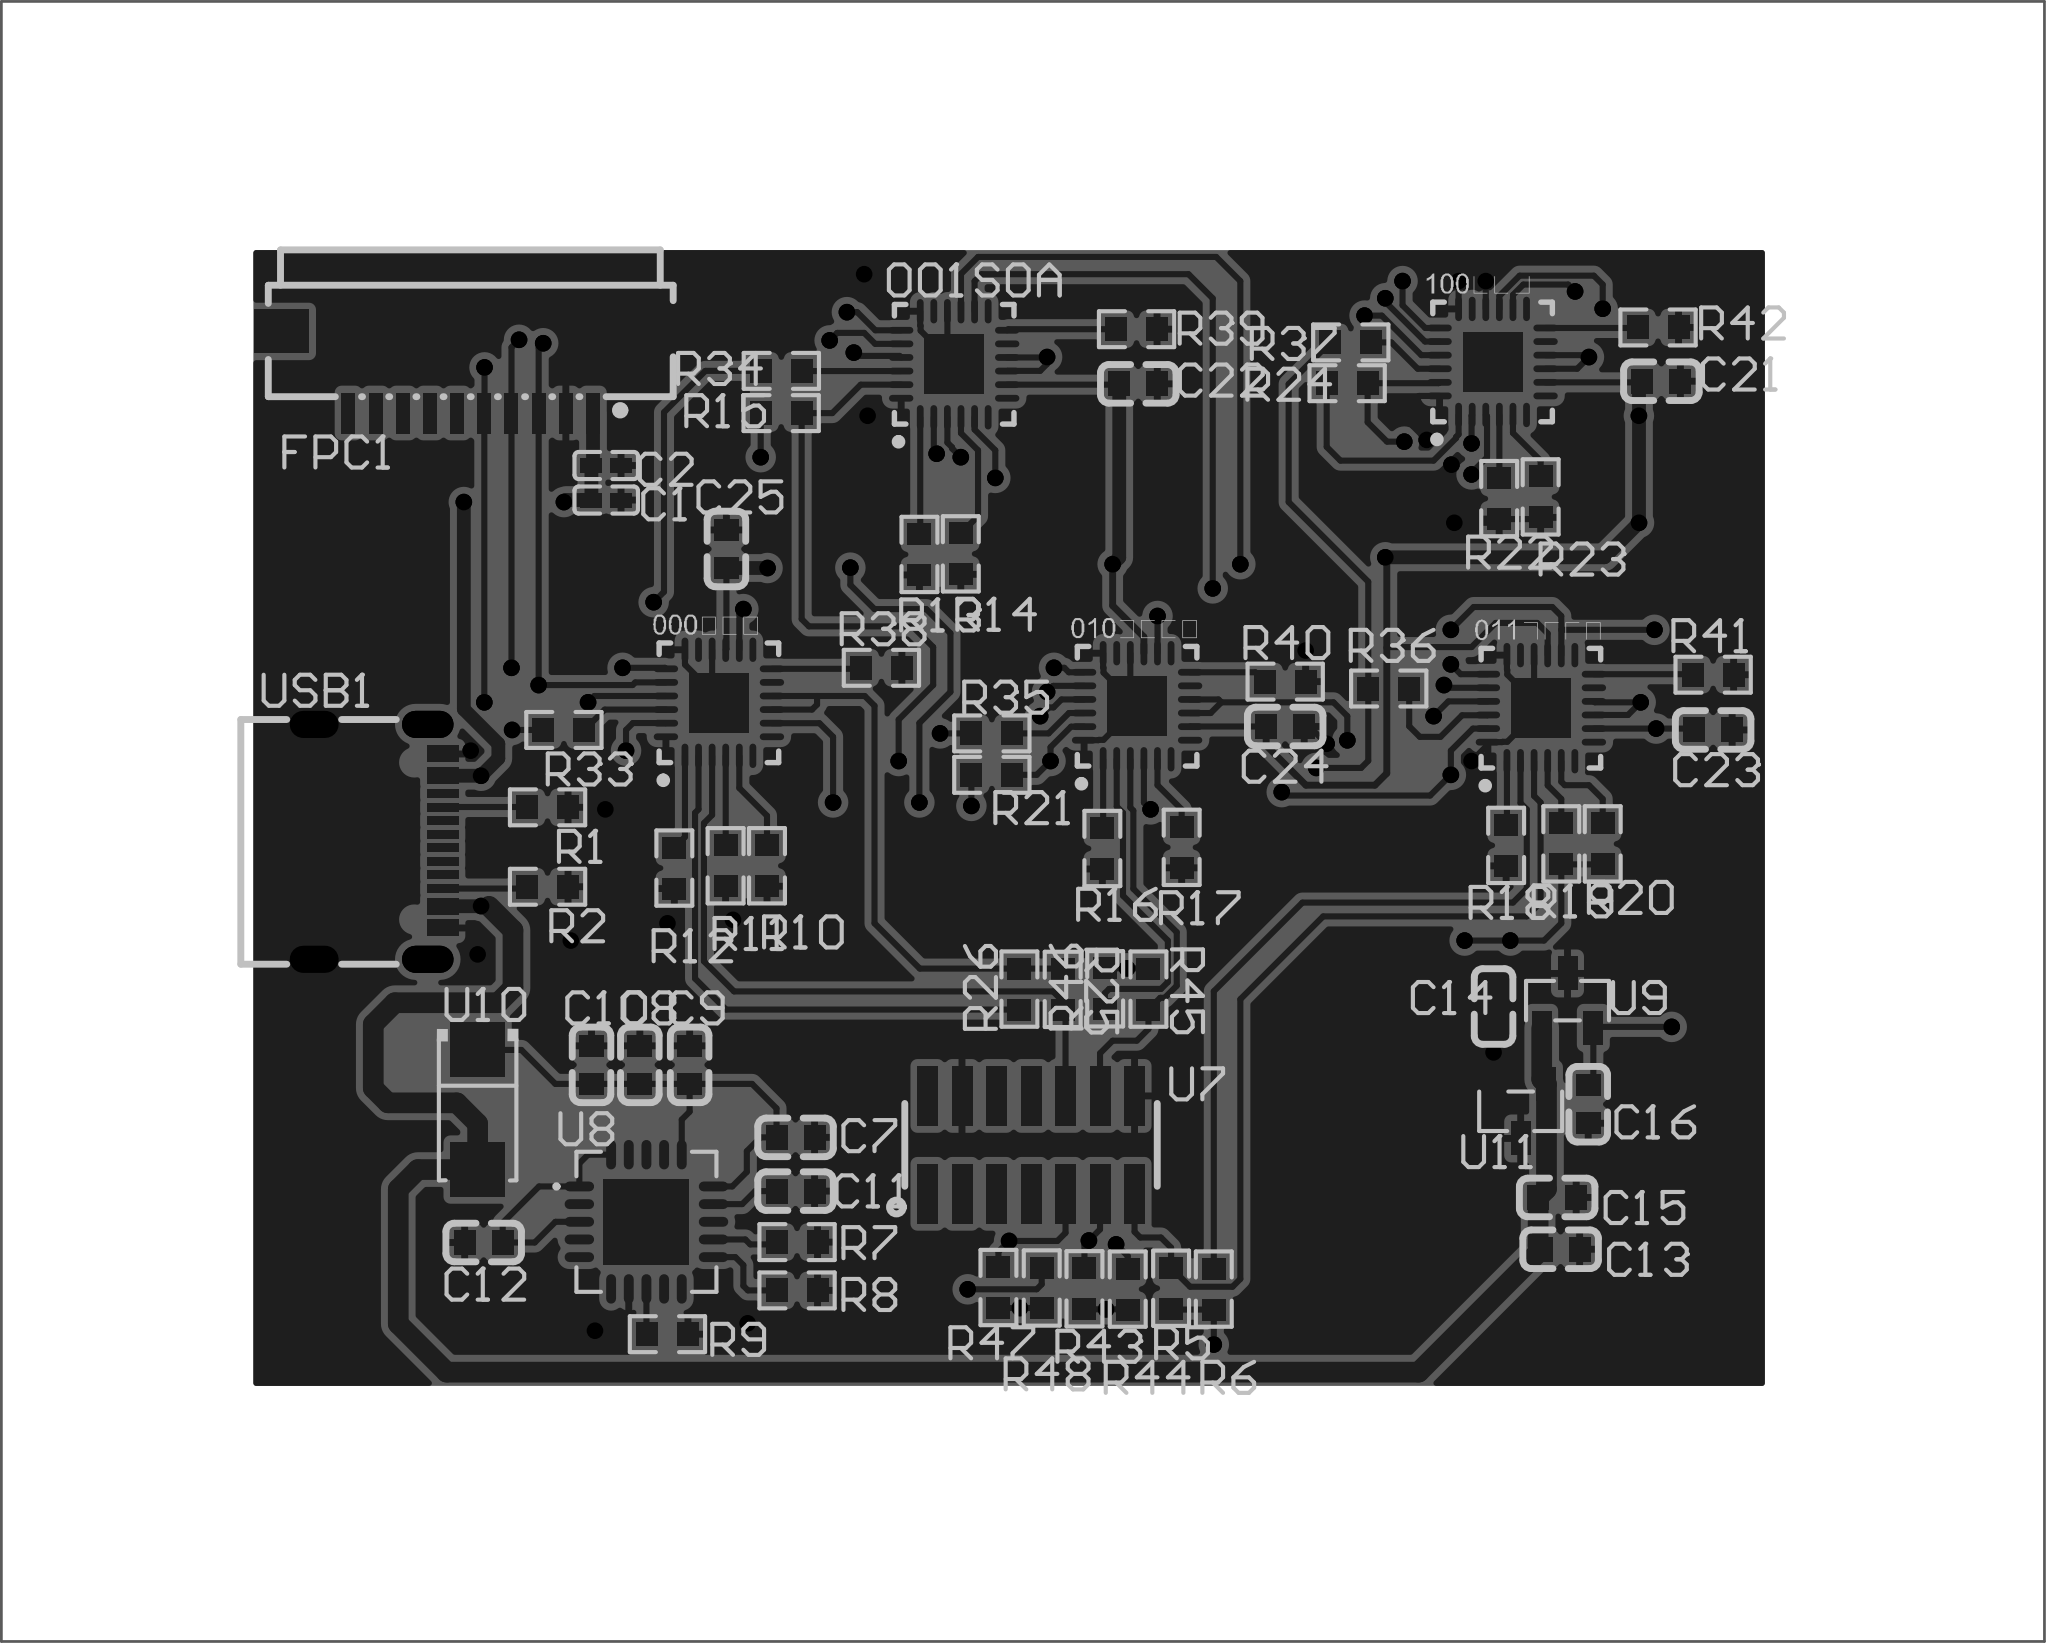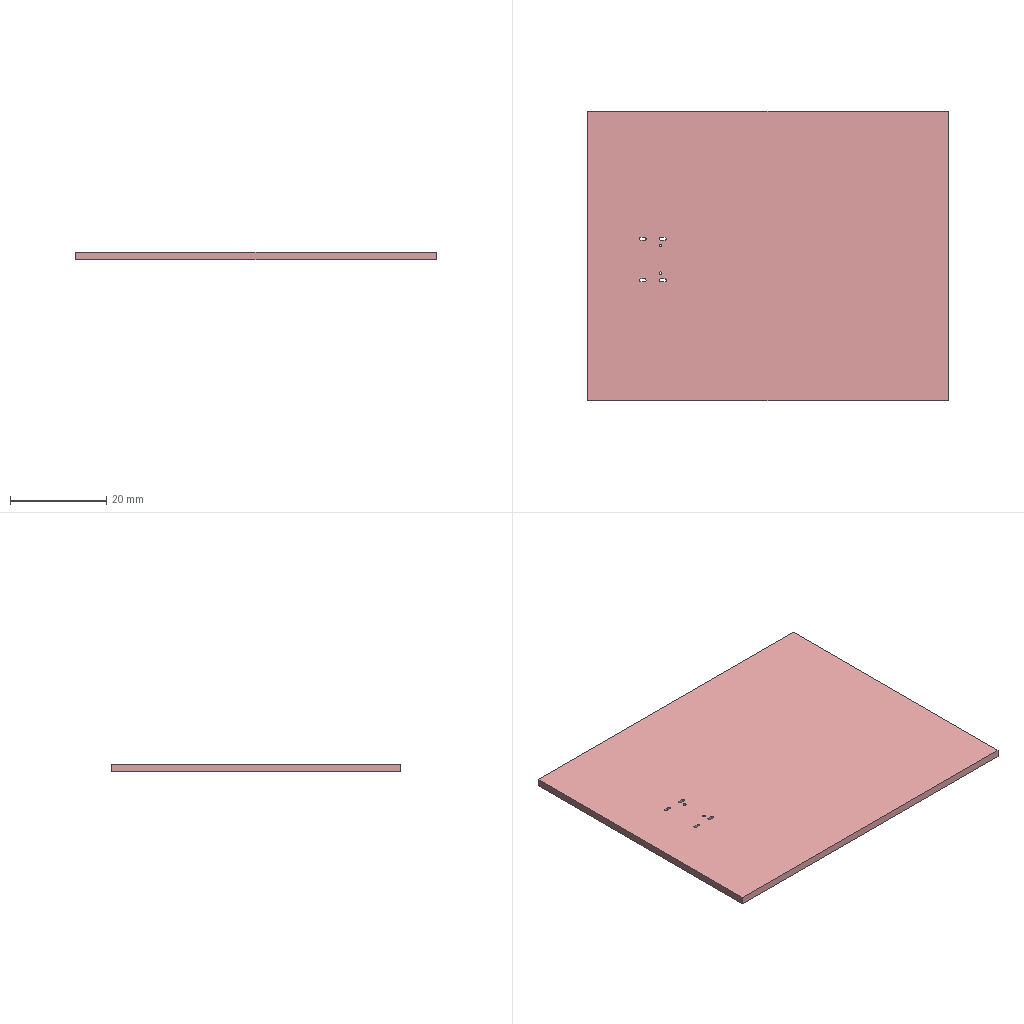Circuit board layout | Altium Designer | box 75.2 x 60.3 x 1.6 mm
Layer stack:
# Altium Designer layer stack of  (unit mm; dielectric type: 0 none, 1 core, 2 prepreg, 3 surface material)
index,name,kind,layer,copper_thickness_mm,dielectric_type,dielectric_thickness_mm,dielectric_material,dielectric_constant
0,Top Paste Mask Layer,other,,,,,,
1,Top Silkscreen Layer,other,,,,,,
2,Top Solder Mask Layer,dielectric,,,3,0.01,,3.3
3,Top Layer,copper,Top Layer,0.035,,,,
4,Dielectric1,dielectric,,,3,1.51,FR4,4.5
5,Bottom Layer,copper,Bottom Layer,0.035,,,,
6,Bottom Solder Mask Layer,dielectric,,,3,0.01,,3.3
7,Bottom Silkscreen Layer,other,,,,,,
8,Bottom Paste Mask Layer,other,,,,,,
# drill layer pairs: low layer,high layer
drill_pair,Top Layer,Bottom Layer
Part placement:
Designator,Comment,Layer,Footprint,Center-X(mm),Center-Y(mm),Rotation
000增益节,ADN8810ACPZ,TopLayer,LFCSP-24_L4.0-W4.0-P0.50-BL-EP2.3,96.255,104.377,0
001SOA,ADN8810ACPZ,TopLayer,LFCSP-24_L4.0-W4.0-P0.50-BL-EP2.3,104.913,116.829,0
010左光栅节,ADN8810ACPZ,TopLayer,LFCSP-24_L4.0-W4.0-P0.50-BL-EP2.3,111.644,104.25,0
011右光栅节,ADN8810ACPZ,TopLayer,LFCSP-24_L4.0-W4.0-P0.50-BL-EP2.3,126.503,104.179,0
100相位节,ADN8810ACPZ,TopLayer,LFCSP-24_L4.0-W4.0-P0.50-BL-EP2.3,124.725,116.914,0
C1,10uF,TopLayer,C0402,92.108,111.835,180
C2,100nF,TopLayer,C0402,92.108,113.105,180
C7,10uF,TopLayer,C0603,99.075,88.392,0
C8,10uF,TopLayer,C0603,93.345,91.059,90
C9,0.1uF,TopLayer,C0603,95.178,91.059,270
C10,0.1uF,TopLayer,C0603,91.567,91.059,270
C11,1uF,TopLayer,C0603,99.075,86.415,180
C12,10uF,TopLayer,C0603,87.598,84.525,0
C13,2.2uF,TopLayer,C0603,127.229,84.277,0
C14,2.2uF,TopLayer,C0603,124.762,93.206,270
C15,2.2uF,TopLayer,C0603,127.102,86.182,0
C16,2.2uF,TopLayer,C0603,128.245,89.611,90
C21,100nF,TopLayer,C0603,130.937,116.205,0
C22,100nF,TopLayer,C0603,111.687,116.109,0
C23,100nF,TopLayer,C0603,132.842,103.378,0
C24,100nF,TopLayer,C0603,117.094,103.505,0
C25,100nF,TopLayer,C0603,96.531,110.034,90
FPC1,Header1X10,TopLayer,FPC-SMD_10P-P1.00_C9900008955,87.122,116.586,180
R1,5.1K,TopLayer,R0603,89.949,100.532,180
R2,5.1K,TopLayer,R0603,89.949,97.611,180
R5,2.2,TopLayer,R0603,112.895,82.843,90
R6,2.2,TopLayer,R0603,114.466,82.812,270
R7,0,TopLayer,R0603,99.13,84.539,0
R8,0,TopLayer,R0603,99.13,82.763,0
R9,0,TopLayer,R0603,94.361,81.153,0
R10,10K,TopLayer,R0603,98.024,98.382,90
R11,10K,TopLayer,R0603,96.5,98.382,90
R12,10K,TopLayer,R0603,94.615,98.298,90
R13,10K,TopLayer,R0603,103.634,109.833,90
R14,10K,TopLayer,R0603,105.156,109.855,90
R15,10K,TopLayer,R0603,98.546,115.031,180
R16,10K,TopLayer,R0603,110.365,99.017,90
R17,10K,TopLayer,R0603,113.284,99.06,90
R18,10K,TopLayer,R0603,125.224,99.131,90
R19,10K,TopLayer,R0603,127.254,99.187,90
R20,10K,TopLayer,R0603,128.778,99.187,90
R21,10K,TopLayer,R0603,106.299,101.727,180
R22,10K,TopLayer,R0603,124.968,111.887,90
R23,10K,TopLayer,R0603,126.494,111.95,90
R24,10K,TopLayer,R0603,119.374,116.132,180
R25,1.37,TopLayer,R0603,108.906,93.835,270
R26,1.37,TopLayer,R0603,107.313,93.846,90
R33,10K,TopLayer,R0603,90.551,103.378,180
R34,10K,TopLayer,R0603,98.552,116.586,180
R35,10K,TopLayer,R0603,106.299,103.251,180
R36,10K,TopLayer,R0603,120.904,104.902,180
R37,10K,TopLayer,R0603,119.507,117.633,180
R38,10K,TopLayer,R0603,102.235,105.664,0
R39,10K,TopLayer,R0603,111.624,118.119,0
R40,10K,TopLayer,R0603,117.094,105.156,0
R41,10K,TopLayer,R0603,132.842,105.41,0
R42,10K,TopLayer,R0603,130.815,118.183,0
R43,2.2,TopLayer,R0603,109.707,82.822,90
R44,2.2,TopLayer,R0603,111.299,82.811,270
R45,2.2,TopLayer,R0603,112.061,93.845,270
R46,2.2,TopLayer,R0603,110.469,93.856,90
R47,1.37,TopLayer,R0603,106.541,82.869,90
R48,1.37,TopLayer,R0603,108.134,82.852,270
U7,ATLS7503,TopLayer,HDR-SMD_14P-P1.27-V-F-R2-C7-LS4.8,107.74,88.116,0
U8,TPS7A4701RGWR,TopLayer,VQFN-20_L5.0-W5.0-P0.65-TL-EP,93.588,85.287,0
U9,REF2930AIDBZT,TopLayer,SOT-23-3_L2.9-W1.3-P1.90-LS2.4-BR,127.483,93.421,270
U10,SS310 Schottky diode SMA,TopLayer,SMA_L4.3-W2.6-LS5.1-R-RD,87.376,89.408,270
U11,REF2940AIDBZT,TopLayer,SOT-23-3_L2.9-W1.3-P1.90-LS2.4-BR,125.759,89.352,90
USB1,Type-C-16P,TopLayer,USB-C-SMD_GT-USB-7010E,83.726,99.262,270
Pad and via stacks:
# Altium Designer via and pad stacks of  (unit mm). Each distinct definition once, with the count of objects using it.
# via: kind,start_layer,end_layer,hole_mm,diameter_mm,mode(0 simple;1 top-mid-bottom;2 full stack),diameter_per_layer,count,example_net
# pad: kind,layer,hole_mm,hole_type(0 round;1 square;2 slot),plating,top_size,top_shape(1 round;2 rect;3 octagon;9 rounded rect),mid_size,bottom_size,mode,footprint,size_per_layer,count,example
pad,Top Layer,0,0,plated,0.9x0.25,1,0.9x0.25,0.9x0.25,0,LFCSP-24_L4.0-W4.0-P0.50-BL-EP2.3,,60,000\u589E\u76CA\u8282.24
pad,Top Layer,0,0,plated,0.25x0.9,1,0.25x0.9,0.25x0.9,0,LFCSP-24_L4.0-W4.0-P0.50-BL-EP2.3,,60,000\u589E\u76CA\u8282.18
pad,Top Layer,0,0,plated,2.2x2.2,2,2.2x2.2,2.2x2.2,0,LFCSP-24_L4.0-W4.0-P0.50-BL-EP2.3,,5,000\u589E\u76CA\u8282.25
pad,Top Layer,0,0,plated,0.7901x0.54,2,0.7901x0.54,0.7901x0.54,0,C0402,,4,C1.2
pad,Top Layer,0,0,plated,0.8x0.9,2,0.8x0.9,0.8x0.9,0,C0603,,30,C7.2
pad,Top Layer,0,0,plated,0.5x1.5,2,0.5x1.5,0.5x1.5,0,FPC-SMD_10P-P1.00_C9900008955,,10,FPC1.1
pad,Top Layer,0,0,plated,2x1.6,2,2x1.6,2x1.6,0,FPC-SMD_10P-P1.00_C9900008955,,2,FPC1.11
pad,Top Layer,0,0,plated,0.8065x0.864,2,0.8065x0.864,0.8065x0.864,0,R0603,,80,R1.2
pad,Top Layer,0,0,plated,2.2x0.74,2,2.2x0.74,2.2x0.74,0,HDR-SMD_14P-P1.27-V-F-R2-C7-LS4.8,,14,U7.1
pad,Top Layer,0,0,plated,1.087x0.364,1,1.087x0.364,1.087x0.364,0,VQFN-20_L5.0-W5.0-P0.65-TL-EP,,10,U8.1
pad,Top Layer,0,0,plated,0.364x1.087,1,0.364x1.087,0.364x1.087,0,VQFN-20_L5.0-W5.0-P0.65-TL-EP,,10,U8.6
pad,Top Layer,0,0,plated,3.15x3.15,2,3.15x3.15,3.15x3.15,0,VQFN-20_L5.0-W5.0-P0.65-TL-EP,,1,U8.21
pad,Top Layer,0,0,plated,1.25x0.7,2,1.25x0.7,1.25x0.7,0,SOT-23-3_L2.9-W1.3-P1.90-LS2.4-BR,,6,U9.1
pad,Top Layer,0,0,plated,2x2,2,2x2,2x2,0,SMA_L4.3-W2.6-LS5.1-R-RD,,2,U10.1
pad,Top Layer,0,0,plated,0.6x1.15,2,0.6x1.15,0.6x1.15,0,USB-C-SMD_GT-USB-7010E,,4,USB1.B1A12
pad,Top Layer,0,0,plated,0.3x1.15,2,0.3x1.15,0.3x1.15,0,USB-C-SMD_GT-USB-7010E,,8,USB1.B5
pad,Multi-Layer,0.6,2,plated,1x1.9,1,1x1.9,1x1.9,0,USB-C-SMD_GT-USB-7010E,,2,USB1.1
pad,Multi-Layer,0.6,2,plated,1x1.8,1,1x1.8,1x1.8,0,USB-C-SMD_GT-USB-7010E,,2,USB1.4
via,Top Layer,Bottom Layer,0.3048,0.61,0,,95,ADN_SPI1_SCK
Copper pours:
name,layer,net,type(0 solid;1 hatched;2 none)
Top Layer-GND,Top Layer,GND,0
Bottom Layer-GND,Bottom Layer,GND,0
Design rules, without the lines most boards share:
# Altium Designer design rules of  (exported by Altium Designer, unit mm)
# columns: name | kind | enabled | priority | scope1 | scope2 | descriptor | typed fields (field=value)
copperRegion | 20 | enabled | 1 | (InNet('GND') OR InNet('IOUT4')) | All | Polygon Connect Rule(Relief Connect )(Conductor Width=10mil) (Relief Angle=90 Angle) (Entries=4) (Air Gap Width=10mil) ((InNet('GND') OR InNet('IOUT4'))),(All) | connect_style(0=relief,1=direct,2=none)=0 relief_conductor_width=0.254 relief_entries=4